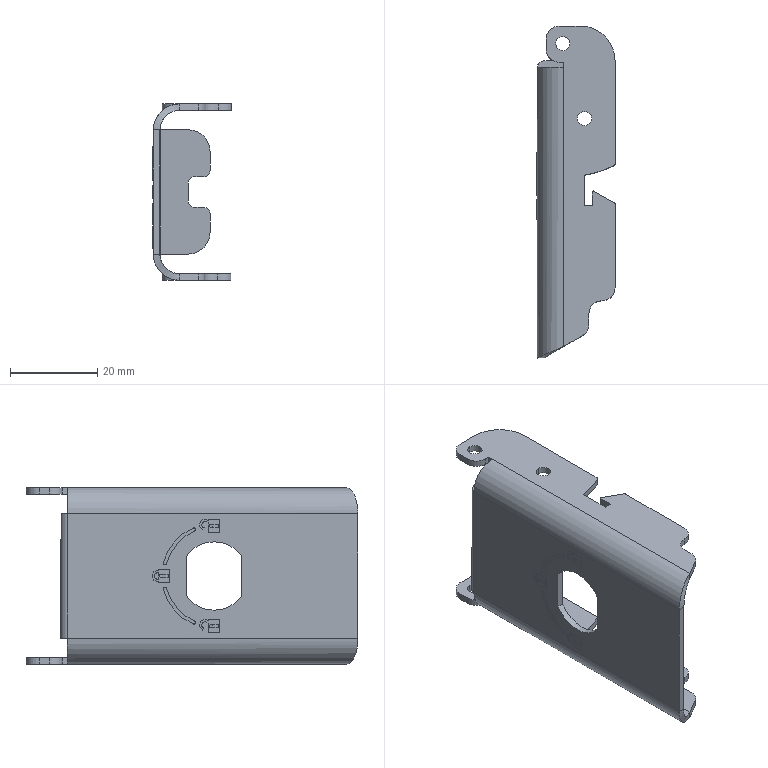Part | SolidWorks | features BaseBody 1 | 1 solid | 162 faces | box 17.928 x 76.116 x 40.539 mm | volume 6929 mm3 | plane 92 | cylinder 68 | spline 2 | commonest cylinder face diameters 6 x10 0.8 x9 3.3 x8 0.75 x6 3 x5 0.4 x4